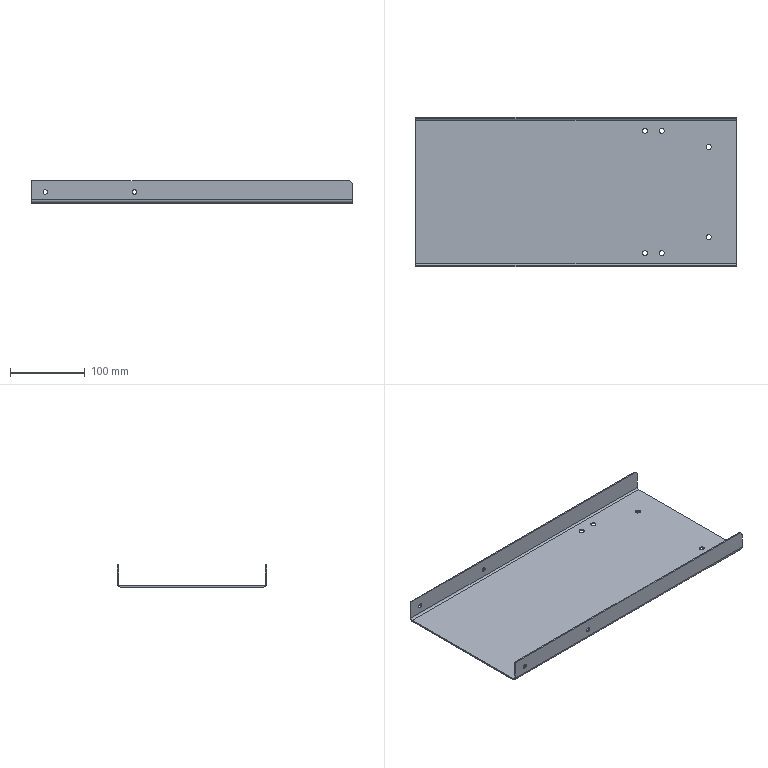Part | STEP file | [01]-13 | 1 solid | 36 faces | box 430 x 200 x 30 mm | volume 173215 mm3 | cylinder 26 | plane 10 | commonest cylinder face diameters 6.8 x12 5.8 x8 4.6 x2 9.2 x2 10 x2